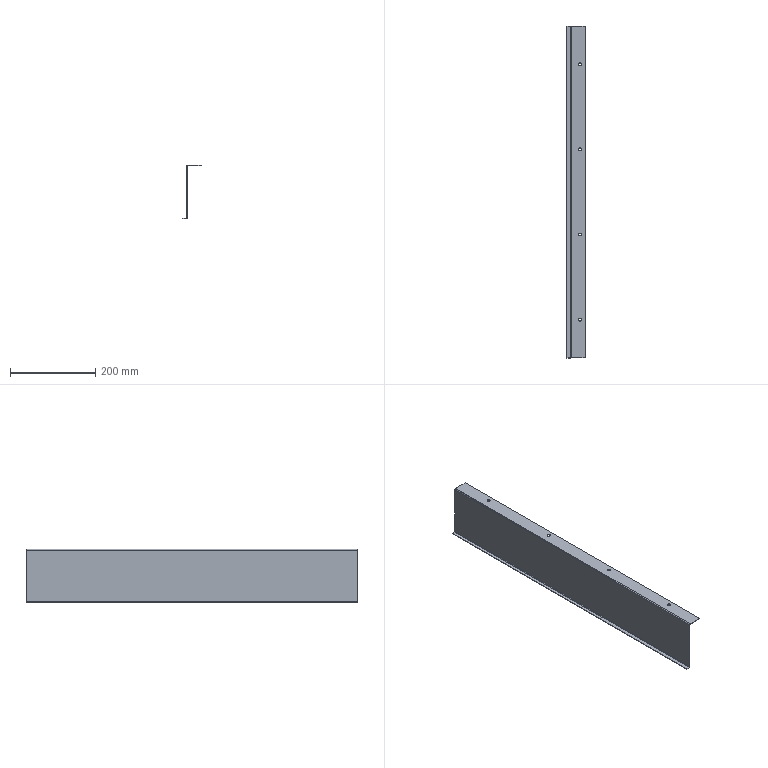Part | STEP file | 1 solid | 30 faces | box 42.8 x 780 x 125 mm | volume 154467 mm3 | plane 18 | cylinder 12 | commonest cylinder face diameters 7 x8 2 x2 4.4 x2